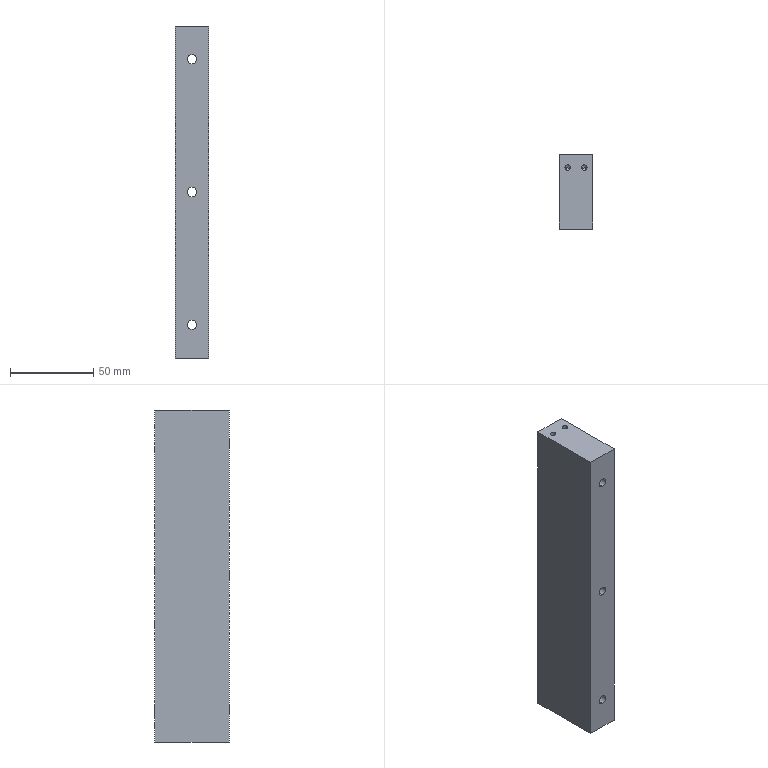Part | STEP file | PN_0079 transport section guide rail pad block A | 1 solid | 53 faces | box 20 x 45 x 200 mm | volume 171286 mm3 | cylinder 28 | cone 16 | plane 9 | commonest cylinder face diameters 2.5 x8 3.3 x8 5.5 x6 10 x6